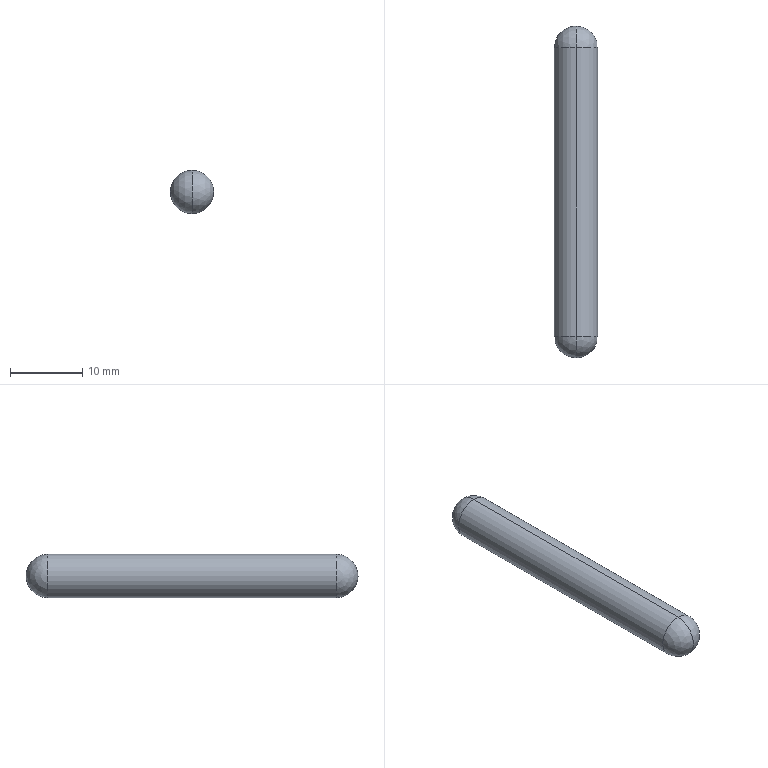Part | SolidWorks | features BaseBody 1 | 1 solid | 6 faces | box 6 x 46 x 6 mm | volume 1244 mm3 | sphere 4 | cylinder 2 | commonest cylinder face diameters 6 x2
STEP:
#1=CARTESIAN_POINT('',(0.,-23.,7.));
#2=VERTEX_POINT('',#1);
#3=CARTESIAN_POINT('',(0.,-20.,10.));
#4=VERTEX_POINT('',#3);
#5=CARTESIAN_POINT('',(0.,-20.,7.));
#6=DIRECTION('',(-1.,0.,0.));
#7=DIRECTION('',(0.,0.,1.));
#8=AXIS2_PLACEMENT_3D('',#5,#6,#7);
#9=CIRCLE('',#8,3.);
#10=EDGE_CURVE('',#2,#4,#9,.T.);
#11=ORIENTED_EDGE('',*,*,#10,.F.);
#12=CARTESIAN_POINT('',(0.,-20.,4.));
#13=VERTEX_POINT('',#12);
#14=CARTESIAN_POINT('',(0.,-20.,7.));
#15=DIRECTION('',(1.,0.,0.));
#16=DIRECTION('',(0.,0.,-1.));
#17=AXIS2_PLACEMENT_3D('',#14,#15,#16);
#18=CIRCLE('',#17,3.);
#19=EDGE_CURVE('',#2,#13,#18,.T.);
#20=ORIENTED_EDGE('',*,*,#19,.T.);
#21=CARTESIAN_POINT('',(0.,-20.,7.));
#22=DIRECTION('',(0.,1.,0.));
#23=DIRECTION('',(0.,0.,1.));
#24=AXIS2_PLACEMENT_3D('',#21,#22,#23);
#25=CIRCLE('',#24,3.);
#26=EDGE_CURVE('',#4,#13,#25,.T.);
#27=ORIENTED_EDGE('',*,*,#26,.F.);
#28=EDGE_LOOP('',(#11,#20,#27));
#29=FACE_OUTER_BOUND('',#28,.T.);
#30=CARTESIAN_POINT('',(0.,-20.,7.));
#31=DIRECTION('',(1.,0.,0.));
#32=DIRECTION('',(0.,0.,1.));
#33=AXIS2_PLACEMENT_3D('',#30,#31,#32);
#34=SPHERICAL_SURFACE('',#33,3.);
#35=ADVANCED_FACE('',(#29),#34,.T.);
#36=CARTESIAN_POINT('',(0.,20.,4.));
#37=VERTEX_POINT('',#36);
#38=CARTESIAN_POINT('',(0.,20.,10.));
#39=VERTEX_POINT('',#38);
#40=CARTESIAN_POINT('',(0.,20.,7.));
#41=DIRECTION('',(0.,1.,0.));
#42=DIRECTION('',(0.,0.,1.));
#43=AXIS2_PLACEMENT_3D('',#40,#41,#42);
#44=CIRCLE('',#43,3.);
#45=EDGE_CURVE('',#37,#39,#44,.T.);
#46=ORIENTED_EDGE('',*,*,#45,.T.);
#47=CARTESIAN_POINT('',(0.,23.,7.));
#48=VERTEX_POINT('',#47);
#49=CARTESIAN_POINT('',(0.,20.,7.));
#50=DIRECTION('',(-1.,0.,0.));
#51=DIRECTION('',(0.,0.,1.));
#52=AXIS2_PLACEMENT_3D('',#49,#50,#51);
#53=CIRCLE('',#52,3.);
#54=EDGE_CURVE('',#39,#48,#53,.T.);
#55=ORIENTED_EDGE('',*,*,#54,.T.);
#56=CARTESIAN_POINT('',(0.,20.,7.));
#57=DIRECTION('',(1.,0.,0.));
#58=DIRECTION('',(0.,0.,-1.));
#59=AXIS2_PLACEMENT_3D('',#56,#57,#58);
#60=CIRCLE('',#59,3.);
#61=EDGE_CURVE('',#37,#48,#60,.T.);
#62=ORIENTED_EDGE('',*,*,#61,.F.);
#63=EDGE_LOOP('',(#46,#55,#62));
#64=FACE_OUTER_BOUND('',#63,.T.);
#65=CARTESIAN_POINT('',(0.,20.,7.));
#66=DIRECTION('',(-1.,0.,0.));
#67=DIRECTION('',(0.,0.,-1.));
#68=AXIS2_PLACEMENT_3D('',#65,#66,#67);
#69=SPHERICAL_SURFACE('',#68,3.);
#70=ADVANCED_FACE('',(#64),#69,.T.);
#71=ORIENTED_EDGE('',*,*,#45,.F.);
#72=CARTESIAN_POINT('',(0.,23.,4.));
#73=DIRECTION('',(0.,-1.,0.));
#74=VECTOR('',#73,1000.);
#75=LINE('',#72,#74);
#76=EDGE_CURVE('',#37,#13,#75,.T.);
#77=ORIENTED_EDGE('',*,*,#76,.T.);
#78=CARTESIAN_POINT('',(0.,-20.,7.));
#79=DIRECTION('',(0.,1.,0.));
#80=DIRECTION('',(0.,0.,1.));
#81=AXIS2_PLACEMENT_3D('',#78,#79,#80);
#82=CIRCLE('',#81,3.);
#83=EDGE_CURVE('',#13,#4,#82,.T.);
#84=ORIENTED_EDGE('',*,*,#83,.T.);
#85=CARTESIAN_POINT('',(0.,23.,10.));
#86=DIRECTION('',(0.,-1.,0.));
#87=VECTOR('',#86,1000.);
#88=LINE('',#85,#87);
#89=EDGE_CURVE('',#39,#4,#88,.T.);
#90=ORIENTED_EDGE('',*,*,#89,.F.);
#91=EDGE_LOOP('',(#71,#77,#84,#90));
#92=FACE_OUTER_BOUND('',#91,.T.);
#93=CARTESIAN_POINT('',(0.,23.,7.));
#94=DIRECTION('',(0.,-1.,0.));
#95=DIRECTION('',(0.,0.,1.));
#96=AXIS2_PLACEMENT_3D('',#93,#94,#95);
#97=CYLINDRICAL_SURFACE('',#96,3.);
#98=ADVANCED_FACE('',(#92),#97,.T.);
#99=ORIENTED_EDGE('',*,*,#76,.F.);
#100=CARTESIAN_POINT('',(0.,20.,7.));
#101=DIRECTION('',(0.,1.,0.));
#102=DIRECTION('',(0.,0.,1.));
#103=AXIS2_PLACEMENT_3D('',#100,#101,#102);
#104=CIRCLE('',#103,3.);
#105=EDGE_CURVE('',#39,#37,#104,.T.);
#106=ORIENTED_EDGE('',*,*,#105,.F.);
#107=ORIENTED_EDGE('',*,*,#89,.T.);
#108=ORIENTED_EDGE('',*,*,#26,.T.);
#109=EDGE_LOOP('',(#99,#106,#107,#108));
#110=FACE_OUTER_BOUND('',#109,.T.);
#111=CARTESIAN_POINT('',(0.,23.,7.));
#112=DIRECTION('',(0.,-1.,0.));
#113=DIRECTION('',(0.,0.,1.));
#114=AXIS2_PLACEMENT_3D('',#111,#112,#113);
#115=CYLINDRICAL_SURFACE('',#114,3.);
#116=ADVANCED_FACE('',(#110),#115,.T.);
#117=ORIENTED_EDGE('',*,*,#54,.F.);
#118=ORIENTED_EDGE('',*,*,#105,.T.);
#119=ORIENTED_EDGE('',*,*,#61,.T.);
#120=EDGE_LOOP('',(#117,#118,#119));
#121=FACE_OUTER_BOUND('',#120,.T.);
#122=CARTESIAN_POINT('',(0.,20.,7.));
#123=DIRECTION('',(-1.,0.,0.));
#124=DIRECTION('',(0.,0.,-1.));
#125=AXIS2_PLACEMENT_3D('',#122,#123,#124);
#126=SPHERICAL_SURFACE('',#125,3.);
#127=ADVANCED_FACE('',(#121),#126,.T.);
#128=ORIENTED_EDGE('',*,*,#19,.F.);
#129=ORIENTED_EDGE('',*,*,#10,.T.);
#130=ORIENTED_EDGE('',*,*,#83,.F.);
#131=EDGE_LOOP('',(#128,#129,#130));
#132=FACE_OUTER_BOUND('',#131,.T.);
#133=CARTESIAN_POINT('',(0.,-20.,7.));
#134=DIRECTION('',(1.,0.,0.));
#135=DIRECTION('',(0.,0.,1.));
#136=AXIS2_PLACEMENT_3D('',#133,#134,#135);
#137=SPHERICAL_SURFACE('',#136,3.);
#138=ADVANCED_FACE('',(#132),#137,.T.);
#139=CLOSED_SHELL('',(#35,#70,#98,#116,#127,#138));
#140=MANIFOLD_SOLID_BREP('',#139);
#141=CARTESIAN_POINT('',(0.,0.,0.));
#142=DIRECTION('',(0.,0.,1.));
#143=DIRECTION('',(1.,0.,0.));
#144=AXIS2_PLACEMENT_3D('',#141,#142,#143);
#145=(LENGTH_UNIT()NAMED_UNIT(*)SI_UNIT(.MILLI.,.METRE.));
#146=UNCERTAINTY_MEASURE_WITH_UNIT(LENGTH_MEASURE(0.00001),#145,'','');
#147=(NAMED_UNIT(*)PLANE_ANGLE_UNIT()SI_UNIT($,.RADIAN.));
#148=(NAMED_UNIT(*)SI_UNIT($,.STERADIAN.)SOLID_ANGLE_UNIT());
#149=(GEOMETRIC_REPRESENTATION_CONTEXT(3)GLOBAL_UNCERTAINTY_ASSIGNED_CONTEXT((#146))GLOBAL_UNIT_ASSIGNED_CONTEXT((#145,#147,#148))REPRESENTATION_CONTEXT('',''));
#150=ADVANCED_BREP_SHAPE_REPRESENTATION('',(#140,#144),#149);